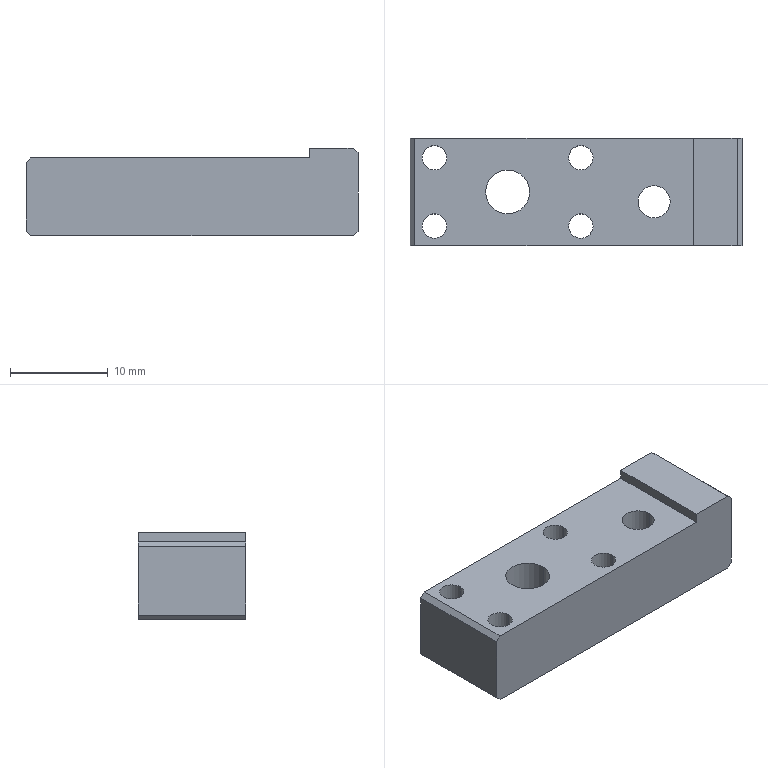Part | STEP file | FBDS-CS-009 | 1 solid | 27 faces | box 34 x 11 x 9 mm | volume 2531 mm3 | cylinder 14 | plane 13 | commonest cylinder face diameters 2.5 x8 3.3 x2 4.5 x2 8 x2
STEP:
#1=CARTESIAN_POINT('',(23.35,-6.5,8.));
#2=VERTEX_POINT('',#1);
#3=CARTESIAN_POINT('',(26.65,-6.5,8.));
#4=VERTEX_POINT('',#3);
#5=CARTESIAN_POINT('',(25.,-6.5,8.));
#6=DIRECTION('',(0.,0.,1.));
#7=DIRECTION('',(1.,0.,0.));
#8=AXIS2_PLACEMENT_3D('',#5,#6,#7);
#9=CIRCLE('',#8,1.65);
#10=EDGE_CURVE('',#2,#4,#9,.T.);
#11=ORIENTED_EDGE('',*,*,#10,.T.);
#12=CARTESIAN_POINT('',(26.65,-6.5,0.));
#13=VERTEX_POINT('',#12);
#14=CARTESIAN_POINT('',(26.65,-6.5,0.));
#15=DIRECTION('',(0.,0.,-1.));
#16=VECTOR('',#15,1000.);
#17=LINE('',#14,#16);
#18=EDGE_CURVE('',#4,#13,#17,.T.);
#19=ORIENTED_EDGE('',*,*,#18,.T.);
#20=CARTESIAN_POINT('',(23.35,-6.5,0.));
#21=VERTEX_POINT('',#20);
#22=CARTESIAN_POINT('',(25.,-6.5,0.));
#23=DIRECTION('',(0.,0.,-1.));
#24=DIRECTION('',(-1.,0.,0.));
#25=AXIS2_PLACEMENT_3D('',#22,#23,#24);
#26=CIRCLE('',#25,1.65);
#27=EDGE_CURVE('',#13,#21,#26,.T.);
#28=ORIENTED_EDGE('',*,*,#27,.T.);
#29=CARTESIAN_POINT('',(23.35,-6.5,0.));
#30=DIRECTION('',(0.,0.,-1.));
#31=VECTOR('',#30,1000.);
#32=LINE('',#29,#31);
#33=EDGE_CURVE('',#2,#21,#32,.T.);
#34=ORIENTED_EDGE('',*,*,#33,.F.);
#35=EDGE_LOOP('',(#11,#19,#28,#34));
#36=FACE_OUTER_BOUND('',#35,.T.);
#37=CARTESIAN_POINT('',(25.,-6.5,0.));
#38=DIRECTION('',(0.,0.,-1.));
#39=DIRECTION('',(-1.,0.,0.));
#40=AXIS2_PLACEMENT_3D('',#37,#38,#39);
#41=CYLINDRICAL_SURFACE('',#40,1.65);
#42=ADVANCED_FACE('',(#36),#41,.F.);
#43=CARTESIAN_POINT('',(14.,-5.5,4.6));
#44=VERTEX_POINT('',#43);
#45=CARTESIAN_POINT('',(6.,-5.5,4.6));
#46=VERTEX_POINT('',#45);
#47=CARTESIAN_POINT('',(10.,-5.5,4.6));
#48=DIRECTION('',(0.,0.,-1.));
#49=DIRECTION('',(-1.,0.,0.));
#50=AXIS2_PLACEMENT_3D('',#47,#48,#49);
#51=CIRCLE('',#50,4.);
#52=EDGE_CURVE('',#44,#46,#51,.T.);
#53=ORIENTED_EDGE('',*,*,#52,.F.);
#54=CARTESIAN_POINT('',(14.,-5.5,0.));
#55=VERTEX_POINT('',#54);
#56=CARTESIAN_POINT('',(14.,-5.5,0.));
#57=DIRECTION('',(0.,0.,-1.));
#58=VECTOR('',#57,1000.);
#59=LINE('',#56,#58);
#60=EDGE_CURVE('',#44,#55,#59,.T.);
#61=ORIENTED_EDGE('',*,*,#60,.T.);
#62=CARTESIAN_POINT('',(6.,-5.5,0.));
#63=VERTEX_POINT('',#62);
#64=CARTESIAN_POINT('',(10.,-5.5,0.));
#65=DIRECTION('',(0.,0.,-1.));
#66=DIRECTION('',(-1.,0.,0.));
#67=AXIS2_PLACEMENT_3D('',#64,#65,#66);
#68=CIRCLE('',#67,4.);
#69=EDGE_CURVE('',#55,#63,#68,.T.);
#70=ORIENTED_EDGE('',*,*,#69,.T.);
#71=CARTESIAN_POINT('',(6.,-5.5,0.));
#72=DIRECTION('',(0.,0.,-1.));
#73=VECTOR('',#72,1000.);
#74=LINE('',#71,#73);
#75=EDGE_CURVE('',#46,#63,#74,.T.);
#76=ORIENTED_EDGE('',*,*,#75,.F.);
#77=EDGE_LOOP('',(#53,#61,#70,#76));
#78=FACE_OUTER_BOUND('',#77,.T.);
#79=CARTESIAN_POINT('',(10.,-5.5,0.));
#80=DIRECTION('',(0.,0.,-1.));
#81=DIRECTION('',(-1.,0.,0.));
#82=AXIS2_PLACEMENT_3D('',#79,#80,#81);
#83=CYLINDRICAL_SURFACE('',#82,4.);
#84=ADVANCED_FACE('',(#78),#83,.F.);
#85=CARTESIAN_POINT('',(7.75,-5.5,8.));
#86=VERTEX_POINT('',#85);
#87=CARTESIAN_POINT('',(12.25,-5.5,8.));
#88=VERTEX_POINT('',#87);
#89=CARTESIAN_POINT('',(10.,-5.5,8.));
#90=DIRECTION('',(0.,0.,1.));
#91=DIRECTION('',(1.,0.,0.));
#92=AXIS2_PLACEMENT_3D('',#89,#90,#91);
#93=CIRCLE('',#92,2.25);
#94=EDGE_CURVE('',#86,#88,#93,.T.);
#95=ORIENTED_EDGE('',*,*,#94,.T.);
#96=CARTESIAN_POINT('',(12.25,-5.5,4.6));
#97=VERTEX_POINT('',#96);
#98=CARTESIAN_POINT('',(12.25,-5.5,0.));
#99=DIRECTION('',(0.,0.,-1.));
#100=VECTOR('',#99,1000.);
#101=LINE('',#98,#100);
#102=EDGE_CURVE('',#88,#97,#101,.T.);
#103=ORIENTED_EDGE('',*,*,#102,.T.);
#104=CARTESIAN_POINT('',(7.75,-5.5,4.6));
#105=VERTEX_POINT('',#104);
#106=CARTESIAN_POINT('',(10.,-5.5,4.6));
#107=DIRECTION('',(0.,0.,-1.));
#108=DIRECTION('',(-1.,0.,0.));
#109=AXIS2_PLACEMENT_3D('',#106,#107,#108);
#110=CIRCLE('',#109,2.25);
#111=EDGE_CURVE('',#97,#105,#110,.T.);
#112=ORIENTED_EDGE('',*,*,#111,.T.);
#113=CARTESIAN_POINT('',(7.75,-5.5,0.));
#114=DIRECTION('',(0.,0.,-1.));
#115=VECTOR('',#114,1000.);
#116=LINE('',#113,#115);
#117=EDGE_CURVE('',#86,#105,#116,.T.);
#118=ORIENTED_EDGE('',*,*,#117,.F.);
#119=EDGE_LOOP('',(#95,#103,#112,#118));
#120=FACE_OUTER_BOUND('',#119,.T.);
#121=CARTESIAN_POINT('',(10.,-5.5,0.));
#122=DIRECTION('',(0.,0.,-1.));
#123=DIRECTION('',(-1.,0.,0.));
#124=AXIS2_PLACEMENT_3D('',#121,#122,#123);
#125=CYLINDRICAL_SURFACE('',#124,2.25);
#126=ADVANCED_FACE('',(#120),#125,.F.);
#127=CARTESIAN_POINT('',(18.75,-2.,8.));
#128=VERTEX_POINT('',#127);
#129=CARTESIAN_POINT('',(16.25,-2.,8.));
#130=VERTEX_POINT('',#129);
#131=CARTESIAN_POINT('',(17.5,-2.,8.));
#132=DIRECTION('',(0.,0.,-1.));
#133=DIRECTION('',(-1.,0.,0.));
#134=AXIS2_PLACEMENT_3D('',#131,#132,#133);
#135=CIRCLE('',#134,1.25);
#136=EDGE_CURVE('',#128,#130,#135,.T.);
#137=ORIENTED_EDGE('',*,*,#136,.F.);
#138=CARTESIAN_POINT('',(18.75,-2.,0.));
#139=VERTEX_POINT('',#138);
#140=CARTESIAN_POINT('',(18.75,-2.,0.));
#141=DIRECTION('',(0.,0.,-1.));
#142=VECTOR('',#141,1000.);
#143=LINE('',#140,#142);
#144=EDGE_CURVE('',#128,#139,#143,.T.);
#145=ORIENTED_EDGE('',*,*,#144,.T.);
#146=CARTESIAN_POINT('',(16.25,-2.,0.));
#147=VERTEX_POINT('',#146);
#148=CARTESIAN_POINT('',(17.5,-2.,0.));
#149=DIRECTION('',(0.,0.,-1.));
#150=DIRECTION('',(-1.,0.,0.));
#151=AXIS2_PLACEMENT_3D('',#148,#149,#150);
#152=CIRCLE('',#151,1.25);
#153=EDGE_CURVE('',#139,#147,#152,.T.);
#154=ORIENTED_EDGE('',*,*,#153,.T.);
#155=CARTESIAN_POINT('',(16.25,-2.,0.));
#156=DIRECTION('',(0.,0.,-1.));
#157=VECTOR('',#156,1000.);
#158=LINE('',#155,#157);
#159=EDGE_CURVE('',#130,#147,#158,.T.);
#160=ORIENTED_EDGE('',*,*,#159,.F.);
#161=EDGE_LOOP('',(#137,#145,#154,#160));
#162=FACE_OUTER_BOUND('',#161,.T.);
#163=CARTESIAN_POINT('',(17.5,-2.,0.));
#164=DIRECTION('',(0.,0.,-1.));
#165=DIRECTION('',(-1.,0.,0.));
#166=AXIS2_PLACEMENT_3D('',#163,#164,#165);
#167=CYLINDRICAL_SURFACE('',#166,1.25);
#168=ADVANCED_FACE('',(#162),#167,.F.);
#169=CARTESIAN_POINT('',(18.75,-9.,8.));
#170=VERTEX_POINT('',#169);
#171=CARTESIAN_POINT('',(16.25,-9.,8.));
#172=VERTEX_POINT('',#171);
#173=CARTESIAN_POINT('',(17.5,-9.,8.));
#174=DIRECTION('',(0.,0.,-1.));
#175=DIRECTION('',(-1.,0.,0.));
#176=AXIS2_PLACEMENT_3D('',#173,#174,#175);
#177=CIRCLE('',#176,1.25);
#178=EDGE_CURVE('',#170,#172,#177,.T.);
#179=ORIENTED_EDGE('',*,*,#178,.F.);
#180=CARTESIAN_POINT('',(18.75,-9.,0.));
#181=VERTEX_POINT('',#180);
#182=CARTESIAN_POINT('',(18.75,-9.,0.));
#183=DIRECTION('',(0.,0.,-1.));
#184=VECTOR('',#183,1000.);
#185=LINE('',#182,#184);
#186=EDGE_CURVE('',#170,#181,#185,.T.);
#187=ORIENTED_EDGE('',*,*,#186,.T.);
#188=CARTESIAN_POINT('',(16.25,-9.,0.));
#189=VERTEX_POINT('',#188);
#190=CARTESIAN_POINT('',(17.5,-9.,0.));
#191=DIRECTION('',(0.,0.,-1.));
#192=DIRECTION('',(-1.,0.,0.));
#193=AXIS2_PLACEMENT_3D('',#190,#191,#192);
#194=CIRCLE('',#193,1.25);
#195=EDGE_CURVE('',#181,#189,#194,.T.);
#196=ORIENTED_EDGE('',*,*,#195,.T.);
#197=CARTESIAN_POINT('',(16.25,-9.,0.));
#198=DIRECTION('',(0.,0.,-1.));
#199=VECTOR('',#198,1000.);
#200=LINE('',#197,#199);
#201=EDGE_CURVE('',#172,#189,#200,.T.);
#202=ORIENTED_EDGE('',*,*,#201,.F.);
#203=EDGE_LOOP('',(#179,#187,#196,#202));
#204=FACE_OUTER_BOUND('',#203,.T.);
#205=CARTESIAN_POINT('',(17.5,-9.,0.));
#206=DIRECTION('',(0.,0.,-1.));
#207=DIRECTION('',(-1.,0.,0.));
#208=AXIS2_PLACEMENT_3D('',#205,#206,#207);
#209=CYLINDRICAL_SURFACE('',#208,1.25);
#210=ADVANCED_FACE('',(#204),#209,.F.);
#211=CARTESIAN_POINT('',(3.75,-9.,8.));
#212=VERTEX_POINT('',#211);
#213=CARTESIAN_POINT('',(1.25,-9.,8.));
#214=VERTEX_POINT('',#213);
#215=CARTESIAN_POINT('',(2.5,-9.,8.));
#216=DIRECTION('',(0.,0.,-1.));
#217=DIRECTION('',(-1.,0.,0.));
#218=AXIS2_PLACEMENT_3D('',#215,#216,#217);
#219=CIRCLE('',#218,1.25);
#220=EDGE_CURVE('',#212,#214,#219,.T.);
#221=ORIENTED_EDGE('',*,*,#220,.F.);
#222=CARTESIAN_POINT('',(3.75,-9.,0.));
#223=VERTEX_POINT('',#222);
#224=CARTESIAN_POINT('',(3.75,-9.,0.));
#225=DIRECTION('',(0.,0.,-1.));
#226=VECTOR('',#225,1000.);
#227=LINE('',#224,#226);
#228=EDGE_CURVE('',#212,#223,#227,.T.);
#229=ORIENTED_EDGE('',*,*,#228,.T.);
#230=CARTESIAN_POINT('',(1.25,-9.,0.));
#231=VERTEX_POINT('',#230);
#232=CARTESIAN_POINT('',(2.5,-9.,0.));
#233=DIRECTION('',(0.,0.,-1.));
#234=DIRECTION('',(-1.,0.,0.));
#235=AXIS2_PLACEMENT_3D('',#232,#233,#234);
#236=CIRCLE('',#235,1.25);
#237=EDGE_CURVE('',#223,#231,#236,.T.);
#238=ORIENTED_EDGE('',*,*,#237,.T.);
#239=CARTESIAN_POINT('',(1.25,-9.,0.));
#240=DIRECTION('',(0.,0.,-1.));
#241=VECTOR('',#240,1000.);
#242=LINE('',#239,#241);
#243=EDGE_CURVE('',#214,#231,#242,.T.);
#244=ORIENTED_EDGE('',*,*,#243,.F.);
#245=EDGE_LOOP('',(#221,#229,#238,#244));
#246=FACE_OUTER_BOUND('',#245,.T.);
#247=CARTESIAN_POINT('',(2.5,-9.,0.));
#248=DIRECTION('',(0.,0.,-1.));
#249=DIRECTION('',(-1.,0.,0.));
#250=AXIS2_PLACEMENT_3D('',#247,#248,#249);
#251=CYLINDRICAL_SURFACE('',#250,1.25);
#252=ADVANCED_FACE('',(#246),#251,.F.);
#253=CARTESIAN_POINT('',(3.75,-2.,8.));
#254=VERTEX_POINT('',#253);
#255=CARTESIAN_POINT('',(1.25,-2.,8.));
#256=VERTEX_POINT('',#255);
#257=CARTESIAN_POINT('',(2.5,-2.,8.));
#258=DIRECTION('',(0.,0.,-1.));
#259=DIRECTION('',(-1.,0.,0.));
#260=AXIS2_PLACEMENT_3D('',#257,#258,#259);
#261=CIRCLE('',#260,1.25);
#262=EDGE_CURVE('',#254,#256,#261,.T.);
#263=ORIENTED_EDGE('',*,*,#262,.F.);
#264=CARTESIAN_POINT('',(3.75,-2.,0.));
#265=VERTEX_POINT('',#264);
#266=CARTESIAN_POINT('',(3.75,-2.,0.));
#267=DIRECTION('',(0.,0.,-1.));
#268=VECTOR('',#267,1000.);
#269=LINE('',#266,#268);
#270=EDGE_CURVE('',#254,#265,#269,.T.);
#271=ORIENTED_EDGE('',*,*,#270,.T.);
#272=CARTESIAN_POINT('',(1.25,-2.,0.));
#273=VERTEX_POINT('',#272);
#274=CARTESIAN_POINT('',(2.5,-2.,0.));
#275=DIRECTION('',(0.,0.,-1.));
#276=DIRECTION('',(-1.,0.,0.));
#277=AXIS2_PLACEMENT_3D('',#274,#275,#276);
#278=CIRCLE('',#277,1.25);
#279=EDGE_CURVE('',#265,#273,#278,.T.);
#280=ORIENTED_EDGE('',*,*,#279,.T.);
#281=CARTESIAN_POINT('',(1.25,-2.,0.));
#282=DIRECTION('',(0.,0.,-1.));
#283=VECTOR('',#282,1000.);
#284=LINE('',#281,#283);
#285=EDGE_CURVE('',#256,#273,#284,.T.);
#286=ORIENTED_EDGE('',*,*,#285,.F.);
#287=EDGE_LOOP('',(#263,#271,#280,#286));
#288=FACE_OUTER_BOUND('',#287,.T.);
#289=CARTESIAN_POINT('',(2.5,-2.,0.));
#290=DIRECTION('',(0.,0.,-1.));
#291=DIRECTION('',(-1.,0.,0.));
#292=AXIS2_PLACEMENT_3D('',#289,#290,#291);
#293=CYLINDRICAL_SURFACE('',#292,1.25);
#294=ADVANCED_FACE('',(#288),#293,.F.);
#295=CARTESIAN_POINT('',(0.,0.,7.5));
#296=VERTEX_POINT('',#295);
#297=CARTESIAN_POINT('',(0.,0.,0.5));
#298=VERTEX_POINT('',#297);
#299=CARTESIAN_POINT('',(0.,0.,8.));
#300=DIRECTION('',(0.,0.,-1.));
#301=VECTOR('',#300,1000.);
#302=LINE('',#299,#301);
#303=EDGE_CURVE('',#296,#298,#302,.T.);
#304=ORIENTED_EDGE('',*,*,#303,.T.);
#305=CARTESIAN_POINT('',(0.,-11.,0.5));
#306=VERTEX_POINT('',#305);
#307=CARTESIAN_POINT('',(0.,0.,0.5));
#308=DIRECTION('',(0.,-1.,0.));
#309=VECTOR('',#308,1000.);
#310=LINE('',#307,#309);
#311=EDGE_CURVE('',#298,#306,#310,.T.);
#312=ORIENTED_EDGE('',*,*,#311,.T.);
#313=CARTESIAN_POINT('',(0.,-11.,7.5));
#314=VERTEX_POINT('',#313);
#315=CARTESIAN_POINT('',(0.,-11.,8.));
#316=DIRECTION('',(0.,0.,-1.));
#317=VECTOR('',#316,1000.);
#318=LINE('',#315,#317);
#319=EDGE_CURVE('',#314,#306,#318,.T.);
#320=ORIENTED_EDGE('',*,*,#319,.F.);
#321=CARTESIAN_POINT('',(0.,0.,7.5));
#322=DIRECTION('',(0.,1.,0.));
#323=VECTOR('',#322,1000.);
#324=LINE('',#321,#323);
#325=EDGE_CURVE('',#314,#296,#324,.T.);
#326=ORIENTED_EDGE('',*,*,#325,.T.);
#327=EDGE_LOOP('',(#304,#312,#320,#326));
#328=FACE_OUTER_BOUND('',#327,.T.);
#329=CARTESIAN_POINT('',(0.,0.,8.));
#330=DIRECTION('',(1.,0.,0.));
#331=DIRECTION('',(0.,0.,-1.));
#332=AXIS2_PLACEMENT_3D('',#329,#330,#331);
#333=PLANE('',#332);
#334=ADVANCED_FACE('',(#328),#333,.F.);
#335=CARTESIAN_POINT('',(34.,-11.,8.5));
#336=VERTEX_POINT('',#335);
#337=CARTESIAN_POINT('',(34.,-11.,0.5));
#338=VERTEX_POINT('',#337);
#339=CARTESIAN_POINT('',(34.,-11.,8.));
#340=DIRECTION('',(0.,0.,-1.));
#341=VECTOR('',#340,1000.);
#342=LINE('',#339,#341);
#343=EDGE_CURVE('',#336,#338,#342,.T.);
#344=ORIENTED_EDGE('',*,*,#343,.F.);
#345=CARTESIAN_POINT('',(33.5,-11.,9.));
#346=VERTEX_POINT('',#345);
#347=CARTESIAN_POINT('',(33.5,-11.,9.));
#348=DIRECTION('',(-0.7071,0.,0.7071));
#349=VECTOR('',#348,1000.);
#350=LINE('',#347,#349);
#351=EDGE_CURVE('',#336,#346,#350,.T.);
#352=ORIENTED_EDGE('',*,*,#351,.T.);
#353=CARTESIAN_POINT('',(29.,-11.,9.));
#354=VERTEX_POINT('',#353);
#355=CARTESIAN_POINT('',(34.,-11.,9.));
#356=DIRECTION('',(1.,0.,0.));
#357=VECTOR('',#356,1000.);
#358=LINE('',#355,#357);
#359=EDGE_CURVE('',#354,#346,#358,.T.);
#360=ORIENTED_EDGE('',*,*,#359,.F.);
#361=CARTESIAN_POINT('',(29.,-11.,8.));
#362=VERTEX_POINT('',#361);
#363=CARTESIAN_POINT('',(29.,-11.,9.));
#364=DIRECTION('',(0.,0.,-1.));
#365=VECTOR('',#364,1000.);
#366=LINE('',#363,#365);
#367=EDGE_CURVE('',#354,#362,#366,.T.);
#368=ORIENTED_EDGE('',*,*,#367,.T.);
#369=CARTESIAN_POINT('',(0.5,-11.,8.));
#370=VERTEX_POINT('',#369);
#371=CARTESIAN_POINT('',(0.,-11.,8.));
#372=DIRECTION('',(1.,0.,0.));
#373=VECTOR('',#372,1000.);
#374=LINE('',#371,#373);
#375=EDGE_CURVE('',#370,#362,#374,.T.);
#376=ORIENTED_EDGE('',*,*,#375,.F.);
#377=CARTESIAN_POINT('',(0.5,-11.,8.));
#378=DIRECTION('',(-0.7071,0.,-0.7071));
#379=VECTOR('',#378,1000.);
#380=LINE('',#377,#379);
#381=EDGE_CURVE('',#370,#314,#380,.T.);
#382=ORIENTED_EDGE('',*,*,#381,.T.);
#383=ORIENTED_EDGE('',*,*,#319,.T.);
#384=CARTESIAN_POINT('',(0.5,-11.,0.));
#385=VERTEX_POINT('',#384);
#386=CARTESIAN_POINT('',(0.,-11.,0.5));
#387=DIRECTION('',(0.7071,0.,-0.7071));
#388=VECTOR('',#387,1000.);
#389=LINE('',#386,#388);
#390=EDGE_CURVE('',#306,#385,#389,.T.);
#391=ORIENTED_EDGE('',*,*,#390,.T.);
#392=CARTESIAN_POINT('',(33.5,-11.,0.));
#393=VERTEX_POINT('',#392);
#394=CARTESIAN_POINT('',(0.,-11.,0.));
#395=DIRECTION('',(1.,0.,0.));
#396=VECTOR('',#395,1000.);
#397=LINE('',#394,#396);
#398=EDGE_CURVE('',#385,#393,#397,.T.);
#399=ORIENTED_EDGE('',*,*,#398,.T.);
#400=CARTESIAN_POINT('',(34.,-11.,0.5));
#401=DIRECTION('',(0.7071,0.,0.7071));
#402=VECTOR('',#401,1000.);
#403=LINE('',#400,#402);
#404=EDGE_CURVE('',#393,#338,#403,.T.);
#405=ORIENTED_EDGE('',*,*,#404,.T.);
#406=EDGE_LOOP('',(#344,#352,#360,#368,#376,#382,#383,#391,#399,#405));
#407=FACE_OUTER_BOUND('',#406,.T.);
#408=CARTESIAN_POINT('',(0.,-11.,8.));
#409=DIRECTION('',(0.,1.,0.));
#410=DIRECTION('',(0.,0.,1.));
#411=AXIS2_PLACEMENT_3D('',#408,#409,#410);
#412=PLANE('',#411);
#413=ADVANCED_FACE('',(#407),#412,.F.);
#414=CARTESIAN_POINT('',(34.,0.,8.5));
#415=VERTEX_POINT('',#414);
#416=CARTESIAN_POINT('',(34.,0.,0.5));
#417=VERTEX_POINT('',#416);
#418=CARTESIAN_POINT('',(34.,0.,8.));
#419=DIRECTION('',(0.,0.,-1.));
#420=VECTOR('',#419,1000.);
#421=LINE('',#418,#420);
#422=EDGE_CURVE('',#415,#417,#421,.T.);
#423=ORIENTED_EDGE('',*,*,#422,.F.);
#424=CARTESIAN_POINT('',(34.,0.,8.5));
#425=DIRECTION('',(0.,-1.,0.));
#426=VECTOR('',#425,1000.);
#427=LINE('',#424,#426);
#428=EDGE_CURVE('',#415,#336,#427,.T.);
#429=ORIENTED_EDGE('',*,*,#428,.T.);
#430=ORIENTED_EDGE('',*,*,#343,.T.);
#431=CARTESIAN_POINT('',(34.,0.,0.5));
#432=DIRECTION('',(0.,1.,0.));
#433=VECTOR('',#432,1000.);
#434=LINE('',#431,#433);
#435=EDGE_CURVE('',#338,#417,#434,.T.);
#436=ORIENTED_EDGE('',*,*,#435,.T.);
#437=EDGE_LOOP('',(#423,#429,#430,#436));
#438=FACE_OUTER_BOUND('',#437,.T.);
#439=CARTESIAN_POINT('',(34.,0.,8.));
#440=DIRECTION('',(-1.,0.,0.));
#441=DIRECTION('',(0.,0.,1.));
#442=AXIS2_PLACEMENT_3D('',#439,#440,#441);
#443=PLANE('',#442);
#444=ADVANCED_FACE('',(#438),#443,.F.);
#445=CARTESIAN_POINT('',(33.5,0.,9.));
#446=VERTEX_POINT('',#445);
#447=CARTESIAN_POINT('',(29.,0.,9.));
#448=VERTEX_POINT('',#447);
#449=CARTESIAN_POINT('',(34.,0.,9.));
#450=DIRECTION('',(-1.,0.,0.));
#451=VECTOR('',#450,1000.);
#452=LINE('',#449,#451);
#453=EDGE_CURVE('',#446,#448,#452,.T.);
#454=ORIENTED_EDGE('',*,*,#453,.F.);
#455=CARTESIAN_POINT('',(33.5,0.,9.));
#456=DIRECTION('',(0.7071,0.,-0.7071));
#457=VECTOR('',#456,1000.);
#458=LINE('',#455,#457);
#459=EDGE_CURVE('',#446,#415,#458,.T.);
#460=ORIENTED_EDGE('',*,*,#459,.T.);
#461=ORIENTED_EDGE('',*,*,#422,.T.);
#462=CARTESIAN_POINT('',(33.5,0.,0.));
#463=VERTEX_POINT('',#462);
#464=CARTESIAN_POINT('',(34.,0.,0.5));
#465=DIRECTION('',(-0.7071,0.,-0.7071));
#466=VECTOR('',#465,1000.);
#467=LINE('',#464,#466);
#468=EDGE_CURVE('',#417,#463,#467,.T.);
#469=ORIENTED_EDGE('',*,*,#468,.T.);
#470=CARTESIAN_POINT('',(0.5,0.,0.));
#471=VERTEX_POINT('',#470);
#472=CARTESIAN_POINT('',(0.,0.,0.));
#473=DIRECTION('',(-1.,0.,0.));
#474=VECTOR('',#473,1000.);
#475=LINE('',#472,#474);
#476=EDGE_CURVE('',#463,#471,#475,.T.);
#477=ORIENTED_EDGE('',*,*,#476,.T.);
#478=CARTESIAN_POINT('',(0.,0.,0.5));
#479=DIRECTION('',(-0.7071,0.,0.7071));
#480=VECTOR('',#479,1000.);
#481=LINE('',#478,#480);
#482=EDGE_CURVE('',#471,#298,#481,.T.);
#483=ORIENTED_EDGE('',*,*,#482,.T.);
#484=ORIENTED_EDGE('',*,*,#303,.F.);
#485=CARTESIAN_POINT('',(0.5,0.,8.));
#486=VERTEX_POINT('',#485);
#487=CARTESIAN_POINT('',(0.5,0.,8.));
#488=DIRECTION('',(0.7071,0.,0.7071));
#489=VECTOR('',#488,1000.);
#490=LINE('',#487,#489);
#491=EDGE_CURVE('',#296,#486,#490,.T.);
#492=ORIENTED_EDGE('',*,*,#491,.T.);
#493=CARTESIAN_POINT('',(29.,0.,8.));
#494=VERTEX_POINT('',#493);
#495=CARTESIAN_POINT('',(0.,0.,8.));
#496=DIRECTION('',(-1.,0.,0.));
#497=VECTOR('',#496,1000.);
#498=LINE('',#495,#497);
#499=EDGE_CURVE('',#494,#486,#498,.T.);
#500=ORIENTED_EDGE('',*,*,#499,.F.);
#501=CARTESIAN_POINT('',(29.,0.,9.));
#502=DIRECTION('',(0.,0.,-1.));
#503=VECTOR('',#502,1000.);
#504=LINE('',#501,#503);
#505=EDGE_CURVE('',#448,#494,#504,.T.);
#506=ORIENTED_EDGE('',*,*,#505,.F.);
#507=EDGE_LOOP('',(#454,#460,#461,#469,#477,#483,#484,#492,#500,#506));
#508=FACE_OUTER_BOUND('',#507,.T.);
#509=CARTESIAN_POINT('',(0.,0.,8.));
#510=DIRECTION('',(0.,-1.,0.));
#511=DIRECTION('',(0.,0.,-1.));
#512=AXIS2_PLACEMENT_3D('',#509,#510,#511);
#513=PLANE('',#512);
#514=ADVANCED_FACE('',(#508),#513,.F.);
#515=ORIENTED_EDGE('',*,*,#10,.F.);
#516=CARTESIAN_POINT('',(25.,-6.5,8.));
#517=DIRECTION('',(0.,0.,1.));
#518=DIRECTION('',(1.,0.,0.));
#519=AXIS2_PLACEMENT_3D('',#516,#517,#518);
#520=CIRCLE('',#519,1.65);
#521=EDGE_CURVE('',#4,#2,#520,.T.);
#522=ORIENTED_EDGE('',*,*,#521,.F.);
#523=EDGE_LOOP('',(#515,#522));
#524=FACE_BOUND('',#523,.T.);
#525=ORIENTED_EDGE('',*,*,#499,.T.);
#526=CARTESIAN_POINT('',(0.5,-11.,8.));
#527=DIRECTION('',(0.,-1.,0.));
#528=VECTOR('',#527,1000.);
#529=LINE('',#526,#528);
#530=EDGE_CURVE('',#486,#370,#529,.T.);
#531=ORIENTED_EDGE('',*,*,#530,.T.);
#532=ORIENTED_EDGE('',*,*,#375,.T.);
#533=CARTESIAN_POINT('',(29.,0.,8.));
#534=DIRECTION('',(0.,-1.,0.));
#535=VECTOR('',#534,1000.);
#536=LINE('',#533,#535);
#537=EDGE_CURVE('',#494,#362,#536,.T.);
#538=ORIENTED_EDGE('',*,*,#537,.F.);
#539=EDGE_LOOP('',(#525,#531,#532,#538));
#540=FACE_OUTER_BOUND('',#539,.T.);
#541=ORIENTED_EDGE('',*,*,#94,.F.);
#542=CARTESIAN_POINT('',(10.,-5.5,8.));
#543=DIRECTION('',(0.,0.,1.));
#544=DIRECTION('',(1.,0.,0.));
#545=AXIS2_PLACEMENT_3D('',#542,#543,#544);
#546=CIRCLE('',#545,2.25);
#547=EDGE_CURVE('',#88,#86,#546,.T.);
#548=ORIENTED_EDGE('',*,*,#547,.F.);
#549=EDGE_LOOP('',(#541,#548));
#550=FACE_BOUND('',#549,.T.);
#551=CARTESIAN_POINT('',(17.5,-2.,8.));
#552=DIRECTION('',(0.,0.,-1.));
#553=DIRECTION('',(-1.,0.,0.));
#554=AXIS2_PLACEMENT_3D('',#551,#552,#553);
#555=CIRCLE('',#554,1.25);
#556=EDGE_CURVE('',#130,#128,#555,.T.);
#557=ORIENTED_EDGE('',*,*,#556,.T.);
#558=ORIENTED_EDGE('',*,*,#136,.T.);
#559=EDGE_LOOP('',(#557,#558));
#560=FACE_BOUND('',#559,.T.);
#561=CARTESIAN_POINT('',(17.5,-9.,8.));
#562=DIRECTION('',(0.,0.,-1.));
#563=DIRECTION('',(-1.,0.,0.));
#564=AXIS2_PLACEMENT_3D('',#561,#562,#563);
#565=CIRCLE('',#564,1.25);
#566=EDGE_CURVE('',#172,#170,#565,.T.);
#567=ORIENTED_EDGE('',*,*,#566,.T.);
#568=ORIENTED_EDGE('',*,*,#178,.T.);
#569=EDGE_LOOP('',(#567,#568));
#570=FACE_BOUND('',#569,.T.);
#571=CARTESIAN_POINT('',(2.5,-9.,8.));
#572=DIRECTION('',(0.,0.,-1.));
#573=DIRECTION('',(-1.,0.,0.));
#574=AXIS2_PLACEMENT_3D('',#571,#572,#573);
#575=CIRCLE('',#574,1.25);
#576=EDGE_CURVE('',#214,#212,#575,.T.);
#577=ORIENTED_EDGE('',*,*,#576,.T.);
#578=ORIENTED_EDGE('',*,*,#220,.T.);
#579=EDGE_LOOP('',(#577,#578));
#580=FACE_BOUND('',#579,.T.);
#581=CARTESIAN_POINT('',(2.5,-2.,8.));
#582=DIRECTION('',(0.,0.,-1.));
#583=DIRECTION('',(-1.,0.,0.));
#584=AXIS2_PLACEMENT_3D('',#581,#582,#583);
#585=CIRCLE('',#584,1.25);
#586=EDGE_CURVE('',#256,#254,#585,.T.);
#587=ORIENTED_EDGE('',*,*,#586,.T.);
#588=ORIENTED_EDGE('',*,*,#262,.T.);
#589=EDGE_LOOP('',(#587,#588));
#590=FACE_BOUND('',#589,.T.);
#591=CARTESIAN_POINT('',(0.,0.,8.));
#592=DIRECTION('',(0.,0.,1.));
#593=DIRECTION('',(1.,0.,0.));
#594=AXIS2_PLACEMENT_3D('',#591,#592,#593);
#595=PLANE('',#594);
#596=ADVANCED_FACE('',(#524,#540,#550,#560,#570,#580,#590),#595,.T.);
#597=CARTESIAN_POINT('',(25.,-6.5,0.));
#598=DIRECTION('',(0.,0.,-1.));
#599=DIRECTION('',(-1.,0.,0.));
#600=AXIS2_PLACEMENT_3D('',#597,#598,#599);
#601=CIRCLE('',#600,1.65);
#602=EDGE_CURVE('',#21,#13,#601,.T.);
#603=ORIENTED_EDGE('',*,*,#602,.F.);
#604=ORIENTED_EDGE('',*,*,#27,.F.);
#605=EDGE_LOOP('',(#603,#604));
#606=FACE_BOUND('',#605,.T.);
#607=CARTESIAN_POINT('',(10.,-5.5,0.));
#608=DIRECTION('',(0.,0.,-1.));
#609=DIRECTION('',(-1.,0.,0.));
#610=AXIS2_PLACEMENT_3D('',#607,#608,#609);
#611=CIRCLE('',#610,4.);
#612=EDGE_CURVE('',#63,#55,#611,.T.);
#613=ORIENTED_EDGE('',*,*,#612,.F.);
#614=ORIENTED_EDGE('',*,*,#69,.F.);
#615=EDGE_LOOP('',(#613,#614));
#616=FACE_BOUND('',#615,.T.);
#617=CARTESIAN_POINT('',(17.5,-2.,0.));
#618=DIRECTION('',(0.,0.,-1.));
#619=DIRECTION('',(-1.,0.,0.));
#620=AXIS2_PLACEMENT_3D('',#617,#618,#619);
#621=CIRCLE('',#620,1.25);
#622=EDGE_CURVE('',#147,#139,#621,.T.);
#623=ORIENTED_EDGE('',*,*,#622,.F.);
#624=ORIENTED_EDGE('',*,*,#153,.F.);
#625=EDGE_LOOP('',(#623,#624));
#626=FACE_BOUND('',#625,.T.);
#627=CARTESIAN_POINT('',(17.5,-9.,0.));
#628=DIRECTION('',(0.,0.,-1.));
#629=DIRECTION('',(-1.,0.,0.));
#630=AXIS2_PLACEMENT_3D('',#627,#628,#629);
#631=CIRCLE('',#630,1.25);
#632=EDGE_CURVE('',#189,#181,#631,.T.);
#633=ORIENTED_EDGE('',*,*,#632,.F.);
#634=ORIENTED_EDGE('',*,*,#195,.F.);
#635=EDGE_LOOP('',(#633,#634));
#636=FACE_BOUND('',#635,.T.);
#637=CARTESIAN_POINT('',(2.5,-9.,0.));
#638=DIRECTION('',(0.,0.,-1.));
#639=DIRECTION('',(-1.,0.,0.));
#640=AXIS2_PLACEMENT_3D('',#637,#638,#639);
#641=CIRCLE('',#640,1.25);
#642=EDGE_CURVE('',#231,#223,#641,.T.);
#643=ORIENTED_EDGE('',*,*,#642,.F.);
#644=ORIENTED_EDGE('',*,*,#237,.F.);
#645=EDGE_LOOP('',(#643,#644));
#646=FACE_BOUND('',#645,.T.);
#647=CARTESIAN_POINT('',(2.5,-2.,0.));
#648=DIRECTION('',(0.,0.,-1.));
#649=DIRECTION('',(-1.,0.,0.));
#650=AXIS2_PLACEMENT_3D('',#647,#648,#649);
#651=CIRCLE('',#650,1.25);
#652=EDGE_CURVE('',#273,#265,#651,.T.);
#653=ORIENTED_EDGE('',*,*,#652,.F.);
#654=ORIENTED_EDGE('',*,*,#279,.F.);
#655=EDGE_LOOP('',(#653,#654));
#656=FACE_BOUND('',#655,.T.);
#657=ORIENTED_EDGE('',*,*,#476,.F.);
#658=CARTESIAN_POINT('',(33.5,0.,0.));
#659=DIRECTION('',(0.,-1.,0.));
#660=VECTOR('',#659,1000.);
#661=LINE('',#658,#660);
#662=EDGE_CURVE('',#463,#393,#661,.T.);
#663=ORIENTED_EDGE('',*,*,#662,.T.);
#664=ORIENTED_EDGE('',*,*,#398,.F.);
#665=CARTESIAN_POINT('',(0.5,0.,0.));
#666=DIRECTION('',(0.,1.,0.));
#667=VECTOR('',#666,1000.);
#668=LINE('',#665,#667);
#669=EDGE_CURVE('',#385,#471,#668,.T.);
#670=ORIENTED_EDGE('',*,*,#669,.T.);
#671=EDGE_LOOP('',(#657,#663,#664,#670));
#672=FACE_OUTER_BOUND('',#671,.T.);
#673=CARTESIAN_POINT('',(0.,0.,0.));
#674=DIRECTION('',(0.,0.,1.));
#675=DIRECTION('',(1.,0.,0.));
#676=AXIS2_PLACEMENT_3D('',#673,#674,#675);
#677=PLANE('',#676);
#678=ADVANCED_FACE('',(#606,#616,#626,#636,#646,#656,#672),#677,.F.);
#679=ORIENTED_EDGE('',*,*,#270,.F.);
#680=ORIENTED_EDGE('',*,*,#586,.F.);
#681=ORIENTED_EDGE('',*,*,#285,.T.);
#682=ORIENTED_EDGE('',*,*,#652,.T.);
#683=EDGE_LOOP('',(#679,#680,#681,#682));
#684=FACE_OUTER_BOUND('',#683,.T.);
#685=CARTESIAN_POINT('',(2.5,-2.,0.));
#686=DIRECTION('',(0.,0.,-1.));
#687=DIRECTION('',(-1.,0.,0.));
#688=AXIS2_PLACEMENT_3D('',#685,#686,#687);
#689=CYLINDRICAL_SURFACE('',#688,1.25);
#690=ADVANCED_FACE('',(#684),#689,.F.);
#691=ORIENTED_EDGE('',*,*,#228,.F.);
#692=ORIENTED_EDGE('',*,*,#576,.F.);
#693=ORIENTED_EDGE('',*,*,#243,.T.);
#694=ORIENTED_EDGE('',*,*,#642,.T.);
#695=EDGE_LOOP('',(#691,#692,#693,#694));
#696=FACE_OUTER_BOUND('',#695,.T.);
#697=CARTESIAN_POINT('',(2.5,-9.,0.));
#698=DIRECTION('',(0.,0.,-1.));
#699=DIRECTION('',(-1.,0.,0.));
#700=AXIS2_PLACEMENT_3D('',#697,#698,#699);
#701=CYLINDRICAL_SURFACE('',#700,1.25);
#702=ADVANCED_FACE('',(#696),#701,.F.);
#703=ORIENTED_EDGE('',*,*,#186,.F.);
#704=ORIENTED_EDGE('',*,*,#566,.F.);
#705=ORIENTED_EDGE('',*,*,#201,.T.);
#706=ORIENTED_EDGE('',*,*,#632,.T.);
#707=EDGE_LOOP('',(#703,#704,#705,#706));
#708=FACE_OUTER_BOUND('',#707,.T.);
#709=CARTESIAN_POINT('',(17.5,-9.,0.));
#710=DIRECTION('',(0.,0.,-1.));
#711=DIRECTION('',(-1.,0.,0.));
#712=AXIS2_PLACEMENT_3D('',#709,#710,#711);
#713=CYLINDRICAL_SURFACE('',#712,1.25);
#714=ADVANCED_FACE('',(#708),#713,.F.);
#715=ORIENTED_EDGE('',*,*,#144,.F.);
#716=ORIENTED_EDGE('',*,*,#556,.F.);
#717=ORIENTED_EDGE('',*,*,#159,.T.);
#718=ORIENTED_EDGE('',*,*,#622,.T.);
#719=EDGE_LOOP('',(#715,#716,#717,#718));
#720=FACE_OUTER_BOUND('',#719,.T.);
#721=CARTESIAN_POINT('',(17.5,-2.,0.));
#722=DIRECTION('',(0.,0.,-1.));
#723=DIRECTION('',(-1.,0.,0.));
#724=AXIS2_PLACEMENT_3D('',#721,#722,#723);
#725=CYLINDRICAL_SURFACE('',#724,1.25);
#726=ADVANCED_FACE('',(#720),#725,.F.);
#727=ORIENTED_EDGE('',*,*,#102,.F.);
#728=ORIENTED_EDGE('',*,*,#547,.T.);
#729=ORIENTED_EDGE('',*,*,#117,.T.);
#730=CARTESIAN_POINT('',(10.,-5.5,4.6));
#731=DIRECTION('',(0.,0.,-1.));
#732=DIRECTION('',(-1.,0.,0.));
#733=AXIS2_PLACEMENT_3D('',#730,#731,#732);
#734=CIRCLE('',#733,2.25);
#735=EDGE_CURVE('',#105,#97,#734,.T.);
#736=ORIENTED_EDGE('',*,*,#735,.T.);
#737=EDGE_LOOP('',(#727,#728,#729,#736));
#738=FACE_OUTER_BOUND('',#737,.T.);
#739=CARTESIAN_POINT('',(10.,-5.5,0.));
#740=DIRECTION('',(0.,0.,-1.));
#741=DIRECTION('',(-1.,0.,0.));
#742=AXIS2_PLACEMENT_3D('',#739,#740,#741);
#743=CYLINDRICAL_SURFACE('',#742,2.25);
#744=ADVANCED_FACE('',(#738),#743,.F.);
#745=ORIENTED_EDGE('',*,*,#735,.F.);
#746=ORIENTED_EDGE('',*,*,#111,.F.);
#747=EDGE_LOOP('',(#745,#746));
#748=FACE_BOUND('',#747,.T.);
#749=CARTESIAN_POINT('',(10.,-5.5,4.6));
#750=DIRECTION('',(0.,0.,-1.));
#751=DIRECTION('',(-1.,0.,0.));
#752=AXIS2_PLACEMENT_3D('',#749,#750,#751);
#753=CIRCLE('',#752,4.);
#754=EDGE_CURVE('',#46,#44,#753,.T.);
#755=ORIENTED_EDGE('',*,*,#754,.T.);
#756=ORIENTED_EDGE('',*,*,#52,.T.);
#757=EDGE_LOOP('',(#755,#756));
#758=FACE_OUTER_BOUND('',#757,.T.);
#759=CARTESIAN_POINT('',(12.25,-5.5,4.6));
#760=DIRECTION('',(0.,0.,1.));
#761=DIRECTION('',(1.,0.,0.));
#762=AXIS2_PLACEMENT_3D('',#759,#760,#761);
#763=PLANE('',#762);
#764=ADVANCED_FACE('',(#748,#758),#763,.F.);
#765=ORIENTED_EDGE('',*,*,#60,.F.);
#766=ORIENTED_EDGE('',*,*,#754,.F.);
#767=ORIENTED_EDGE('',*,*,#75,.T.);
#768=ORIENTED_EDGE('',*,*,#612,.T.);
#769=EDGE_LOOP('',(#765,#766,#767,#768));
#770=FACE_OUTER_BOUND('',#769,.T.);
#771=CARTESIAN_POINT('',(10.,-5.5,0.));
#772=DIRECTION('',(0.,0.,-1.));
#773=DIRECTION('',(-1.,0.,0.));
#774=AXIS2_PLACEMENT_3D('',#771,#772,#773);
#775=CYLINDRICAL_SURFACE('',#774,4.);
#776=ADVANCED_FACE('',(#770),#775,.F.);
#777=ORIENTED_EDGE('',*,*,#537,.T.);
#778=ORIENTED_EDGE('',*,*,#367,.F.);
#779=CARTESIAN_POINT('',(29.,0.,9.));
#780=DIRECTION('',(0.,-1.,0.));
#781=VECTOR('',#780,1000.);
#782=LINE('',#779,#781);
#783=EDGE_CURVE('',#448,#354,#782,.T.);
#784=ORIENTED_EDGE('',*,*,#783,.F.);
#785=ORIENTED_EDGE('',*,*,#505,.T.);
#786=EDGE_LOOP('',(#777,#778,#784,#785));
#787=FACE_OUTER_BOUND('',#786,.T.);
#788=CARTESIAN_POINT('',(29.,0.,9.));
#789=DIRECTION('',(1.,0.,0.));
#790=DIRECTION('',(0.,0.,-1.));
#791=AXIS2_PLACEMENT_3D('',#788,#789,#790);
#792=PLANE('',#791);
#793=ADVANCED_FACE('',(#787),#792,.F.);
#794=ORIENTED_EDGE('',*,*,#359,.T.);
#795=CARTESIAN_POINT('',(33.5,0.,9.));
#796=DIRECTION('',(0.,1.,0.));
#797=VECTOR('',#796,1000.);
#798=LINE('',#795,#797);
#799=EDGE_CURVE('',#346,#446,#798,.T.);
#800=ORIENTED_EDGE('',*,*,#799,.T.);
#801=ORIENTED_EDGE('',*,*,#453,.T.);
#802=ORIENTED_EDGE('',*,*,#783,.T.);
#803=EDGE_LOOP('',(#794,#800,#801,#802));
#804=FACE_OUTER_BOUND('',#803,.T.);
#805=CARTESIAN_POINT('',(0.,0.,9.));
#806=DIRECTION('',(0.,0.,-1.));
#807=DIRECTION('',(-1.,0.,0.));
#808=AXIS2_PLACEMENT_3D('',#805,#806,#807);
#809=PLANE('',#808);
#810=ADVANCED_FACE('',(#804),#809,.F.);
#811=ORIENTED_EDGE('',*,*,#351,.F.);
#812=ORIENTED_EDGE('',*,*,#428,.F.);
#813=ORIENTED_EDGE('',*,*,#459,.F.);
#814=ORIENTED_EDGE('',*,*,#799,.F.);
#815=EDGE_LOOP('',(#811,#812,#813,#814));
#816=FACE_OUTER_BOUND('',#815,.T.);
#817=CARTESIAN_POINT('',(33.5,0.,9.));
#818=DIRECTION('',(-0.7071,0.,-0.7071));
#819=DIRECTION('',(0.,1.,0.));
#820=AXIS2_PLACEMENT_3D('',#817,#818,#819);
#821=PLANE('',#820);
#822=ADVANCED_FACE('',(#816),#821,.F.);
#823=ORIENTED_EDGE('',*,*,#404,.F.);
#824=ORIENTED_EDGE('',*,*,#662,.F.);
#825=ORIENTED_EDGE('',*,*,#468,.F.);
#826=ORIENTED_EDGE('',*,*,#435,.F.);
#827=EDGE_LOOP('',(#823,#824,#825,#826));
#828=FACE_OUTER_BOUND('',#827,.T.);
#829=CARTESIAN_POINT('',(34.,0.,0.5));
#830=DIRECTION('',(-0.7071,0.,0.7071));
#831=DIRECTION('',(0.,1.,0.));
#832=AXIS2_PLACEMENT_3D('',#829,#830,#831);
#833=PLANE('',#832);
#834=ADVANCED_FACE('',(#828),#833,.F.);
#835=ORIENTED_EDGE('',*,*,#482,.F.);
#836=ORIENTED_EDGE('',*,*,#669,.F.);
#837=ORIENTED_EDGE('',*,*,#390,.F.);
#838=ORIENTED_EDGE('',*,*,#311,.F.);
#839=EDGE_LOOP('',(#835,#836,#837,#838));
#840=FACE_OUTER_BOUND('',#839,.T.);
#841=CARTESIAN_POINT('',(0.,0.,0.5));
#842=DIRECTION('',(0.7071,0.,0.7071));
#843=DIRECTION('',(0.,-1.,0.));
#844=AXIS2_PLACEMENT_3D('',#841,#842,#843);
#845=PLANE('',#844);
#846=ADVANCED_FACE('',(#840),#845,.F.);
#847=ORIENTED_EDGE('',*,*,#491,.F.);
#848=ORIENTED_EDGE('',*,*,#325,.F.);
#849=ORIENTED_EDGE('',*,*,#381,.F.);
#850=ORIENTED_EDGE('',*,*,#530,.F.);
#851=EDGE_LOOP('',(#847,#848,#849,#850));
#852=FACE_OUTER_BOUND('',#851,.T.);
#853=CARTESIAN_POINT('',(0.5,0.,8.));
#854=DIRECTION('',(-0.7071,0.,0.7071));
#855=DIRECTION('',(0.,1.,0.));
#856=AXIS2_PLACEMENT_3D('',#853,#854,#855);
#857=PLANE('',#856);
#858=ADVANCED_FACE('',(#852),#857,.T.);
#859=ORIENTED_EDGE('',*,*,#18,.F.);
#860=ORIENTED_EDGE('',*,*,#521,.T.);
#861=ORIENTED_EDGE('',*,*,#33,.T.);
#862=ORIENTED_EDGE('',*,*,#602,.T.);
#863=EDGE_LOOP('',(#859,#860,#861,#862));
#864=FACE_OUTER_BOUND('',#863,.T.);
#865=CARTESIAN_POINT('',(25.,-6.5,0.));
#866=DIRECTION('',(0.,0.,-1.));
#867=DIRECTION('',(-1.,0.,0.));
#868=AXIS2_PLACEMENT_3D('',#865,#866,#867);
#869=CYLINDRICAL_SURFACE('',#868,1.65);
#870=ADVANCED_FACE('',(#864),#869,.F.);
#871=CLOSED_SHELL('',(#42,#84,#126,#168,#210,#252,#294,#334,#413,#444,#514,#596,#678,#690,#702,#714,#726,#744,#764,#776,#793,#810,#822,#834,#846,#858,#870));
#872=MANIFOLD_SOLID_BREP('',#871);
#873=CARTESIAN_POINT('',(0.,0.,0.));
#874=DIRECTION('',(0.,0.,1.));
#875=DIRECTION('',(1.,0.,0.));
#876=AXIS2_PLACEMENT_3D('',#873,#874,#875);
#877=(LENGTH_UNIT()NAMED_UNIT(*)SI_UNIT(.MILLI.,.METRE.));
#878=UNCERTAINTY_MEASURE_WITH_UNIT(LENGTH_MEASURE(0.00001),#877,'','');
#879=(NAMED_UNIT(*)PLANE_ANGLE_UNIT()SI_UNIT($,.RADIAN.));
#880=(NAMED_UNIT(*)SI_UNIT($,.STERADIAN.)SOLID_ANGLE_UNIT());
#881=(GEOMETRIC_REPRESENTATION_CONTEXT(3)GLOBAL_UNCERTAINTY_ASSIGNED_CONTEXT((#878))GLOBAL_UNIT_ASSIGNED_CONTEXT((#877,#879,#880))REPRESENTATION_CONTEXT('',''));
#882=ADVANCED_BREP_SHAPE_REPRESENTATION('',(#872,#876),#881);